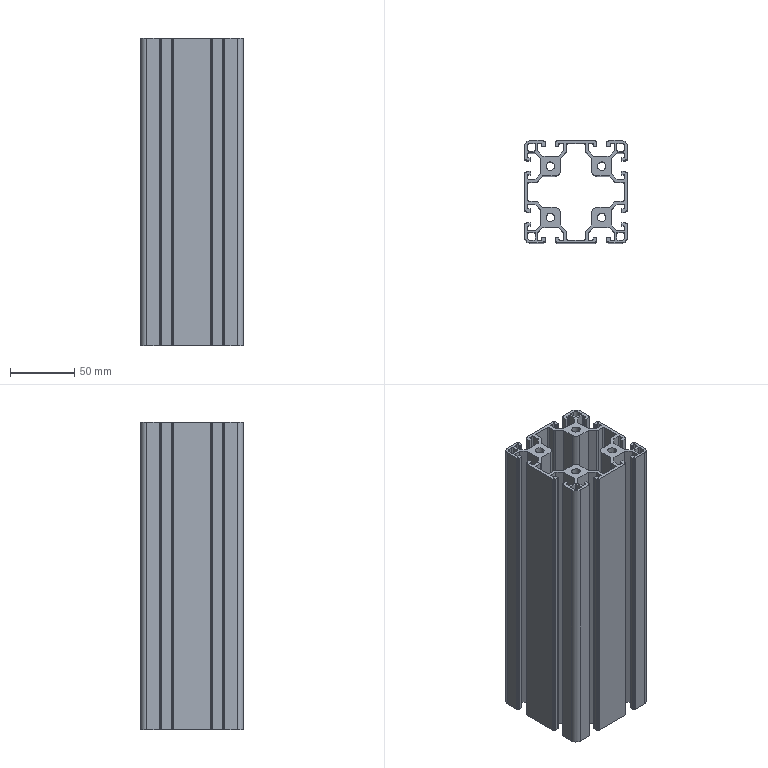Part | STEP file | LE-8-8080-S-OO_LE0313205421 | 1 solid | 380 faces | box 80 x 80 x 240 mm | volume 421917 mm3 | plane 194 | cylinder 186 | commonest cylinder face diameters 0.6 x90 2 x52 0.4 x16 4 x8 6.8 x8 5 x4